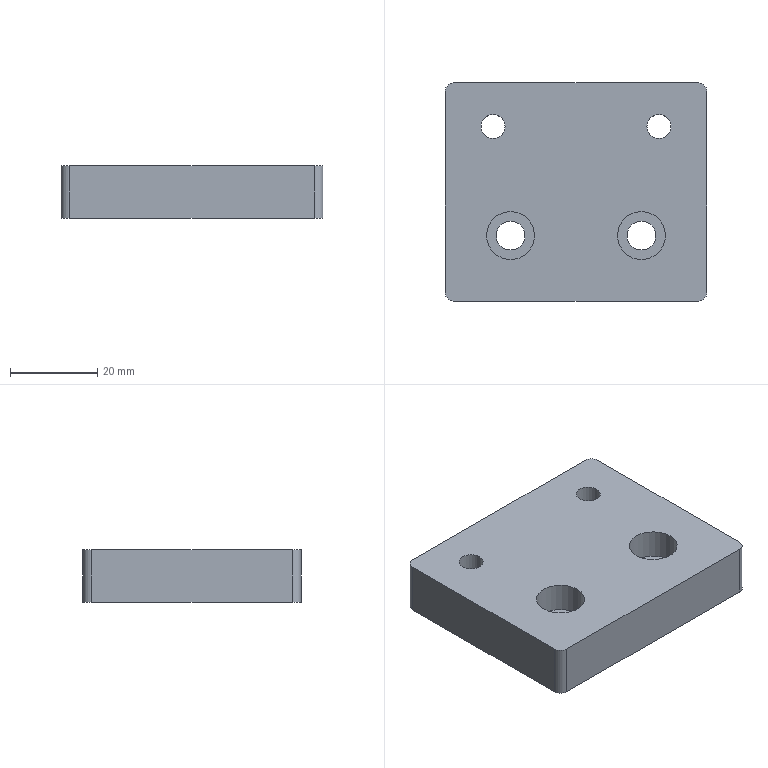Part | STEP file | SynoNew-0304-049 | 1 solid | 22 faces | box 60 x 50 x 12 mm | volume 33116 mm3 | cylinder 12 | plane 10 | commonest cylinder face diameters 4 x4 5.5 x2 6.6 x2 10 x2 11 x2
STEP:
#1=CARTESIAN_POINT('',(-28.,-25.,12.));
#2=VERTEX_POINT('',#1);
#3=CARTESIAN_POINT('',(-30.,-23.,12.));
#4=VERTEX_POINT('',#3);
#5=CARTESIAN_POINT('',(-28.,-23.,12.));
#6=DIRECTION('',(0.,0.,-1.));
#7=DIRECTION('',(-0.7071,-0.7071,0.));
#8=AXIS2_PLACEMENT_3D('',#5,#6,#7);
#9=CIRCLE('',#8,2.);
#10=EDGE_CURVE('',#2,#4,#9,.T.);
#11=ORIENTED_EDGE('',*,*,#10,.T.);
#12=CARTESIAN_POINT('',(-30.,-23.,0.));
#13=VERTEX_POINT('',#12);
#14=CARTESIAN_POINT('',(-30.,-23.,0.));
#15=DIRECTION('',(0.,0.,-1.));
#16=VECTOR('',#15,10.);
#17=LINE('',#14,#16);
#18=EDGE_CURVE('',#4,#13,#17,.T.);
#19=ORIENTED_EDGE('',*,*,#18,.T.);
#20=CARTESIAN_POINT('',(-28.,-25.,0.));
#21=VERTEX_POINT('',#20);
#22=CARTESIAN_POINT('',(-28.,-23.,0.));
#23=DIRECTION('',(0.,0.,1.));
#24=DIRECTION('',(-0.7071,-0.7071,0.));
#25=AXIS2_PLACEMENT_3D('',#22,#23,#24);
#26=CIRCLE('',#25,2.);
#27=EDGE_CURVE('',#13,#21,#26,.T.);
#28=ORIENTED_EDGE('',*,*,#27,.T.);
#29=CARTESIAN_POINT('',(-28.,-25.,0.));
#30=DIRECTION('',(0.,0.,1.));
#31=VECTOR('',#30,10.);
#32=LINE('',#29,#31);
#33=EDGE_CURVE('',#21,#2,#32,.T.);
#34=ORIENTED_EDGE('',*,*,#33,.T.);
#35=EDGE_LOOP('',(#11,#19,#28,#34));
#36=FACE_OUTER_BOUND('',#35,.T.);
#37=CARTESIAN_POINT('',(-28.,-23.,0.));
#38=DIRECTION('',(0.,0.,1.));
#39=DIRECTION('',(-0.7071,-0.7071,0.));
#40=AXIS2_PLACEMENT_3D('',#37,#38,#39);
#41=CYLINDRICAL_SURFACE('',#40,2.);
#42=ADVANCED_FACE('',(#36),#41,.T.);
#43=ORIENTED_EDGE('',*,*,#18,.F.);
#44=CARTESIAN_POINT('',(-30.,23.,12.));
#45=VERTEX_POINT('',#44);
#46=CARTESIAN_POINT('',(-30.,25.,12.));
#47=DIRECTION('',(0.,-1.,0.));
#48=VECTOR('',#47,10.);
#49=LINE('',#46,#48);
#50=EDGE_CURVE('',#45,#4,#49,.T.);
#51=ORIENTED_EDGE('',*,*,#50,.F.);
#52=CARTESIAN_POINT('',(-30.,23.,0.));
#53=VERTEX_POINT('',#52);
#54=CARTESIAN_POINT('',(-30.,23.,0.));
#55=DIRECTION('',(0.,0.,1.));
#56=VECTOR('',#55,10.);
#57=LINE('',#54,#56);
#58=EDGE_CURVE('',#53,#45,#57,.T.);
#59=ORIENTED_EDGE('',*,*,#58,.F.);
#60=CARTESIAN_POINT('',(-30.,25.,0.));
#61=DIRECTION('',(0.,-1.,0.));
#62=VECTOR('',#61,10.);
#63=LINE('',#60,#62);
#64=EDGE_CURVE('',#53,#13,#63,.T.);
#65=ORIENTED_EDGE('',*,*,#64,.T.);
#66=EDGE_LOOP('',(#43,#51,#59,#65));
#67=FACE_OUTER_BOUND('',#66,.T.);
#68=CARTESIAN_POINT('',(-30.,25.,0.));
#69=DIRECTION('',(-1.,0.,0.));
#70=DIRECTION('',(0.,-1.,0.));
#71=AXIS2_PLACEMENT_3D('',#68,#69,#70);
#72=PLANE('',#71);
#73=ADVANCED_FACE('',(#67),#72,.T.);
#74=ORIENTED_EDGE('',*,*,#10,.F.);
#75=CARTESIAN_POINT('',(28.,-25.,12.));
#76=VERTEX_POINT('',#75);
#77=CARTESIAN_POINT('',(-30.,-25.,12.));
#78=DIRECTION('',(1.,0.,0.));
#79=VECTOR('',#78,10.);
#80=LINE('',#77,#79);
#81=EDGE_CURVE('',#2,#76,#80,.T.);
#82=ORIENTED_EDGE('',*,*,#81,.T.);
#83=CARTESIAN_POINT('',(30.,-23.,12.));
#84=VERTEX_POINT('',#83);
#85=CARTESIAN_POINT('',(28.,-23.,12.));
#86=DIRECTION('',(0.,0.,-1.));
#87=DIRECTION('',(0.7071,-0.7071,0.));
#88=AXIS2_PLACEMENT_3D('',#85,#86,#87);
#89=CIRCLE('',#88,2.);
#90=EDGE_CURVE('',#84,#76,#89,.T.);
#91=ORIENTED_EDGE('',*,*,#90,.F.);
#92=CARTESIAN_POINT('',(30.,23.,12.));
#93=VERTEX_POINT('',#92);
#94=CARTESIAN_POINT('',(30.,-25.,12.));
#95=DIRECTION('',(0.,1.,0.));
#96=VECTOR('',#95,10.);
#97=LINE('',#94,#96);
#98=EDGE_CURVE('',#84,#93,#97,.T.);
#99=ORIENTED_EDGE('',*,*,#98,.T.);
#100=CARTESIAN_POINT('',(28.,25.,12.));
#101=VERTEX_POINT('',#100);
#102=CARTESIAN_POINT('',(28.,23.,12.));
#103=DIRECTION('',(0.,0.,-1.));
#104=DIRECTION('',(0.7071,0.7071,0.));
#105=AXIS2_PLACEMENT_3D('',#102,#103,#104);
#106=CIRCLE('',#105,2.);
#107=EDGE_CURVE('',#101,#93,#106,.T.);
#108=ORIENTED_EDGE('',*,*,#107,.F.);
#109=CARTESIAN_POINT('',(-28.,25.,12.));
#110=VERTEX_POINT('',#109);
#111=CARTESIAN_POINT('',(30.,25.,12.));
#112=DIRECTION('',(-1.,0.,0.));
#113=VECTOR('',#112,10.);
#114=LINE('',#111,#113);
#115=EDGE_CURVE('',#101,#110,#114,.T.);
#116=ORIENTED_EDGE('',*,*,#115,.T.);
#117=CARTESIAN_POINT('',(-28.,23.,12.));
#118=DIRECTION('',(0.,0.,-1.));
#119=DIRECTION('',(-0.7071,0.7071,0.));
#120=AXIS2_PLACEMENT_3D('',#117,#118,#119);
#121=CIRCLE('',#120,2.);
#122=EDGE_CURVE('',#45,#110,#121,.T.);
#123=ORIENTED_EDGE('',*,*,#122,.F.);
#124=ORIENTED_EDGE('',*,*,#50,.T.);
#125=EDGE_LOOP('',(#74,#82,#91,#99,#108,#116,#123,#124));
#126=FACE_OUTER_BOUND('',#125,.T.);
#127=CARTESIAN_POINT('',(20.5,-10.,12.));
#128=VERTEX_POINT('',#127);
#129=CARTESIAN_POINT('',(9.5,-10.,12.));
#130=VERTEX_POINT('',#129);
#131=CARTESIAN_POINT('',(15.,-10.,12.));
#132=DIRECTION('',(0.,0.,-1.));
#133=DIRECTION('',(1.,0.,0.));
#134=AXIS2_PLACEMENT_3D('',#131,#132,#133);
#135=CIRCLE('',#134,5.5);
#136=EDGE_CURVE('',#128,#130,#135,.T.);
#137=ORIENTED_EDGE('',*,*,#136,.T.);
#138=CARTESIAN_POINT('',(15.,-10.,12.));
#139=DIRECTION('',(0.,0.,-1.));
#140=DIRECTION('',(1.,0.,0.));
#141=AXIS2_PLACEMENT_3D('',#138,#139,#140);
#142=CIRCLE('',#141,5.5);
#143=EDGE_CURVE('',#130,#128,#142,.T.);
#144=ORIENTED_EDGE('',*,*,#143,.T.);
#145=EDGE_LOOP('',(#137,#144));
#146=FACE_BOUND('',#145,.T.);
#147=CARTESIAN_POINT('',(-9.5,-10.,12.));
#148=VERTEX_POINT('',#147);
#149=CARTESIAN_POINT('',(-20.5,-10.,12.));
#150=VERTEX_POINT('',#149);
#151=CARTESIAN_POINT('',(-15.,-10.,12.));
#152=DIRECTION('',(0.,0.,-1.));
#153=DIRECTION('',(1.,0.,0.));
#154=AXIS2_PLACEMENT_3D('',#151,#152,#153);
#155=CIRCLE('',#154,5.5);
#156=EDGE_CURVE('',#148,#150,#155,.T.);
#157=ORIENTED_EDGE('',*,*,#156,.T.);
#158=CARTESIAN_POINT('',(-15.,-10.,12.));
#159=DIRECTION('',(0.,0.,-1.));
#160=DIRECTION('',(1.,0.,0.));
#161=AXIS2_PLACEMENT_3D('',#158,#159,#160);
#162=CIRCLE('',#161,5.5);
#163=EDGE_CURVE('',#150,#148,#162,.T.);
#164=ORIENTED_EDGE('',*,*,#163,.T.);
#165=EDGE_LOOP('',(#157,#164));
#166=FACE_BOUND('',#165,.T.);
#167=CARTESIAN_POINT('',(-16.25,15.,12.));
#168=VERTEX_POINT('',#167);
#169=CARTESIAN_POINT('',(-19.,15.,12.));
#170=DIRECTION('',(0.,0.,-1.));
#171=DIRECTION('',(-1.,0.,0.));
#172=AXIS2_PLACEMENT_3D('',#169,#170,#171);
#173=CIRCLE('',#172,2.75);
#174=EDGE_CURVE('',#168,#168,#173,.T.);
#175=ORIENTED_EDGE('',*,*,#174,.T.);
#176=EDGE_LOOP('',(#175));
#177=FACE_BOUND('',#176,.T.);
#178=CARTESIAN_POINT('',(21.75,15.,12.));
#179=VERTEX_POINT('',#178);
#180=CARTESIAN_POINT('',(19.,15.,12.));
#181=DIRECTION('',(0.,0.,-1.));
#182=DIRECTION('',(-1.,0.,0.));
#183=AXIS2_PLACEMENT_3D('',#180,#181,#182);
#184=CIRCLE('',#183,2.75);
#185=EDGE_CURVE('',#179,#179,#184,.T.);
#186=ORIENTED_EDGE('',*,*,#185,.T.);
#187=EDGE_LOOP('',(#186));
#188=FACE_BOUND('',#187,.T.);
#189=CARTESIAN_POINT('',(0.,0.,12.));
#190=DIRECTION('',(0.,0.,1.));
#191=DIRECTION('',(1.,0.,0.));
#192=AXIS2_PLACEMENT_3D('',#189,#190,#191);
#193=PLANE('',#192);
#194=ADVANCED_FACE('',(#126,#146,#166,#177,#188),#193,.T.);
#195=ORIENTED_EDGE('',*,*,#90,.T.);
#196=CARTESIAN_POINT('',(28.,-25.,0.));
#197=VERTEX_POINT('',#196);
#198=CARTESIAN_POINT('',(28.,-25.,0.));
#199=DIRECTION('',(0.,0.,-1.));
#200=VECTOR('',#199,10.);
#201=LINE('',#198,#200);
#202=EDGE_CURVE('',#76,#197,#201,.T.);
#203=ORIENTED_EDGE('',*,*,#202,.T.);
#204=CARTESIAN_POINT('',(30.,-23.,0.));
#205=VERTEX_POINT('',#204);
#206=CARTESIAN_POINT('',(28.,-23.,0.));
#207=DIRECTION('',(0.,0.,1.));
#208=DIRECTION('',(0.7071,-0.7071,0.));
#209=AXIS2_PLACEMENT_3D('',#206,#207,#208);
#210=CIRCLE('',#209,2.);
#211=EDGE_CURVE('',#197,#205,#210,.T.);
#212=ORIENTED_EDGE('',*,*,#211,.T.);
#213=CARTESIAN_POINT('',(30.,-23.,0.));
#214=DIRECTION('',(0.,0.,1.));
#215=VECTOR('',#214,10.);
#216=LINE('',#213,#215);
#217=EDGE_CURVE('',#205,#84,#216,.T.);
#218=ORIENTED_EDGE('',*,*,#217,.T.);
#219=EDGE_LOOP('',(#195,#203,#212,#218));
#220=FACE_OUTER_BOUND('',#219,.T.);
#221=CARTESIAN_POINT('',(28.,-23.,0.));
#222=DIRECTION('',(0.,0.,1.));
#223=DIRECTION('',(0.7071,-0.7071,0.));
#224=AXIS2_PLACEMENT_3D('',#221,#222,#223);
#225=CYLINDRICAL_SURFACE('',#224,2.);
#226=ADVANCED_FACE('',(#220),#225,.T.);
#227=ORIENTED_EDGE('',*,*,#217,.F.);
#228=CARTESIAN_POINT('',(30.,23.,0.));
#229=VERTEX_POINT('',#228);
#230=CARTESIAN_POINT('',(30.,-25.,0.));
#231=DIRECTION('',(0.,1.,0.));
#232=VECTOR('',#231,10.);
#233=LINE('',#230,#232);
#234=EDGE_CURVE('',#205,#229,#233,.T.);
#235=ORIENTED_EDGE('',*,*,#234,.T.);
#236=CARTESIAN_POINT('',(30.,23.,0.));
#237=DIRECTION('',(0.,0.,-1.));
#238=VECTOR('',#237,10.);
#239=LINE('',#236,#238);
#240=EDGE_CURVE('',#93,#229,#239,.T.);
#241=ORIENTED_EDGE('',*,*,#240,.F.);
#242=ORIENTED_EDGE('',*,*,#98,.F.);
#243=EDGE_LOOP('',(#227,#235,#241,#242));
#244=FACE_OUTER_BOUND('',#243,.T.);
#245=CARTESIAN_POINT('',(30.,-25.,0.));
#246=DIRECTION('',(1.,0.,0.));
#247=DIRECTION('',(0.,1.,0.));
#248=AXIS2_PLACEMENT_3D('',#245,#246,#247);
#249=PLANE('',#248);
#250=ADVANCED_FACE('',(#244),#249,.T.);
#251=ORIENTED_EDGE('',*,*,#107,.T.);
#252=ORIENTED_EDGE('',*,*,#240,.T.);
#253=CARTESIAN_POINT('',(28.,25.,0.));
#254=VERTEX_POINT('',#253);
#255=CARTESIAN_POINT('',(28.,23.,0.));
#256=DIRECTION('',(0.,0.,1.));
#257=DIRECTION('',(0.7071,0.7071,0.));
#258=AXIS2_PLACEMENT_3D('',#255,#256,#257);
#259=CIRCLE('',#258,2.);
#260=EDGE_CURVE('',#229,#254,#259,.T.);
#261=ORIENTED_EDGE('',*,*,#260,.T.);
#262=CARTESIAN_POINT('',(28.,25.,0.));
#263=DIRECTION('',(0.,0.,1.));
#264=VECTOR('',#263,10.);
#265=LINE('',#262,#264);
#266=EDGE_CURVE('',#254,#101,#265,.T.);
#267=ORIENTED_EDGE('',*,*,#266,.T.);
#268=EDGE_LOOP('',(#251,#252,#261,#267));
#269=FACE_OUTER_BOUND('',#268,.T.);
#270=CARTESIAN_POINT('',(28.,23.,0.));
#271=DIRECTION('',(0.,0.,1.));
#272=DIRECTION('',(0.7071,0.7071,0.));
#273=AXIS2_PLACEMENT_3D('',#270,#271,#272);
#274=CYLINDRICAL_SURFACE('',#273,2.);
#275=ADVANCED_FACE('',(#269),#274,.T.);
#276=ORIENTED_EDGE('',*,*,#122,.T.);
#277=CARTESIAN_POINT('',(-28.,25.,0.));
#278=VERTEX_POINT('',#277);
#279=CARTESIAN_POINT('',(-28.,25.,0.));
#280=DIRECTION('',(0.,0.,-1.));
#281=VECTOR('',#280,10.);
#282=LINE('',#279,#281);
#283=EDGE_CURVE('',#110,#278,#282,.T.);
#284=ORIENTED_EDGE('',*,*,#283,.T.);
#285=CARTESIAN_POINT('',(-28.,23.,0.));
#286=DIRECTION('',(0.,0.,1.));
#287=DIRECTION('',(-0.7071,0.7071,0.));
#288=AXIS2_PLACEMENT_3D('',#285,#286,#287);
#289=CIRCLE('',#288,2.);
#290=EDGE_CURVE('',#278,#53,#289,.T.);
#291=ORIENTED_EDGE('',*,*,#290,.T.);
#292=ORIENTED_EDGE('',*,*,#58,.T.);
#293=EDGE_LOOP('',(#276,#284,#291,#292));
#294=FACE_OUTER_BOUND('',#293,.T.);
#295=CARTESIAN_POINT('',(-28.,23.,0.));
#296=DIRECTION('',(0.,0.,1.));
#297=DIRECTION('',(-0.7071,0.7071,0.));
#298=AXIS2_PLACEMENT_3D('',#295,#296,#297);
#299=CYLINDRICAL_SURFACE('',#298,2.);
#300=ADVANCED_FACE('',(#294),#299,.T.);
#301=CARTESIAN_POINT('',(20.5,-10.,5.2));
#302=VERTEX_POINT('',#301);
#303=CARTESIAN_POINT('',(9.5,-10.,5.2));
#304=VERTEX_POINT('',#303);
#305=CARTESIAN_POINT('',(15.,-10.,5.2));
#306=DIRECTION('',(0.,0.,1.));
#307=DIRECTION('',(1.,0.,0.));
#308=AXIS2_PLACEMENT_3D('',#305,#306,#307);
#309=CIRCLE('',#308,5.5);
#310=EDGE_CURVE('',#302,#304,#309,.T.);
#311=ORIENTED_EDGE('',*,*,#310,.T.);
#312=CARTESIAN_POINT('',(15.,-10.,5.2));
#313=DIRECTION('',(0.,0.,1.));
#314=DIRECTION('',(1.,0.,0.));
#315=AXIS2_PLACEMENT_3D('',#312,#313,#314);
#316=CIRCLE('',#315,5.5);
#317=EDGE_CURVE('',#304,#302,#316,.T.);
#318=ORIENTED_EDGE('',*,*,#317,.T.);
#319=EDGE_LOOP('',(#311,#318));
#320=FACE_OUTER_BOUND('',#319,.T.);
#321=CARTESIAN_POINT('',(11.7,-10.,5.2));
#322=VERTEX_POINT('',#321);
#323=CARTESIAN_POINT('',(15.,-10.,5.2));
#324=DIRECTION('',(0.,0.,1.));
#325=DIRECTION('',(1.,0.,0.));
#326=AXIS2_PLACEMENT_3D('',#323,#324,#325);
#327=CIRCLE('',#326,3.3);
#328=EDGE_CURVE('',#322,#322,#327,.T.);
#329=ORIENTED_EDGE('',*,*,#328,.F.);
#330=EDGE_LOOP('',(#329));
#331=FACE_BOUND('',#330,.T.);
#332=CARTESIAN_POINT('',(15.,-10.,5.2));
#333=DIRECTION('',(0.,0.,1.));
#334=DIRECTION('',(1.,0.,0.));
#335=AXIS2_PLACEMENT_3D('',#332,#333,#334);
#336=PLANE('',#335);
#337=ADVANCED_FACE('',(#320,#331),#336,.T.);
#338=ORIENTED_EDGE('',*,*,#136,.F.);
#339=ORIENTED_EDGE('',*,*,#143,.F.);
#340=CARTESIAN_POINT('',(9.5,-10.,8.6));
#341=DIRECTION('',(0.,0.,-1.));
#342=VECTOR('',#341,5.5);
#343=LINE('',#340,#342);
#344=EDGE_CURVE('',#130,#304,#343,.T.);
#345=ORIENTED_EDGE('',*,*,#344,.T.);
#346=ORIENTED_EDGE('',*,*,#310,.F.);
#347=ORIENTED_EDGE('',*,*,#317,.F.);
#348=ORIENTED_EDGE('',*,*,#344,.F.);
#349=EDGE_LOOP('',(#338,#339,#345,#346,#347,#348));
#350=FACE_OUTER_BOUND('',#349,.T.);
#351=CARTESIAN_POINT('',(15.,-10.,8.6));
#352=DIRECTION('',(0.,0.,1.));
#353=DIRECTION('',(1.,0.,0.));
#354=AXIS2_PLACEMENT_3D('',#351,#352,#353);
#355=CYLINDRICAL_SURFACE('',#354,5.5);
#356=ADVANCED_FACE('',(#350),#355,.F.);
#357=ORIENTED_EDGE('',*,*,#328,.T.);
#358=CARTESIAN_POINT('',(11.7,-10.,0.));
#359=VERTEX_POINT('',#358);
#360=CARTESIAN_POINT('',(11.7,-10.,-67.019));
#361=DIRECTION('',(0.,0.,-1.));
#362=VECTOR('',#361,3.3);
#363=LINE('',#360,#362);
#364=EDGE_CURVE('',#322,#359,#363,.T.);
#365=ORIENTED_EDGE('',*,*,#364,.T.);
#366=CARTESIAN_POINT('',(15.,-10.,0.));
#367=DIRECTION('',(0.,0.,1.));
#368=DIRECTION('',(1.,0.,0.));
#369=AXIS2_PLACEMENT_3D('',#366,#367,#368);
#370=CIRCLE('',#369,3.3);
#371=EDGE_CURVE('',#359,#359,#370,.T.);
#372=ORIENTED_EDGE('',*,*,#371,.F.);
#373=ORIENTED_EDGE('',*,*,#364,.F.);
#374=EDGE_LOOP('',(#357,#365,#372,#373));
#375=FACE_OUTER_BOUND('',#374,.T.);
#376=CARTESIAN_POINT('',(15.,-10.,-67.019));
#377=DIRECTION('',(0.,0.,1.));
#378=DIRECTION('',(1.,0.,0.));
#379=AXIS2_PLACEMENT_3D('',#376,#377,#378);
#380=CYLINDRICAL_SURFACE('',#379,3.3);
#381=ADVANCED_FACE('',(#375),#380,.F.);
#382=CARTESIAN_POINT('',(-9.5,-10.,5.2));
#383=VERTEX_POINT('',#382);
#384=CARTESIAN_POINT('',(-20.5,-10.,5.2));
#385=VERTEX_POINT('',#384);
#386=CARTESIAN_POINT('',(-15.,-10.,5.2));
#387=DIRECTION('',(0.,0.,1.));
#388=DIRECTION('',(1.,0.,0.));
#389=AXIS2_PLACEMENT_3D('',#386,#387,#388);
#390=CIRCLE('',#389,5.5);
#391=EDGE_CURVE('',#383,#385,#390,.T.);
#392=ORIENTED_EDGE('',*,*,#391,.T.);
#393=CARTESIAN_POINT('',(-15.,-10.,5.2));
#394=DIRECTION('',(0.,0.,1.));
#395=DIRECTION('',(1.,0.,0.));
#396=AXIS2_PLACEMENT_3D('',#393,#394,#395);
#397=CIRCLE('',#396,5.5);
#398=EDGE_CURVE('',#385,#383,#397,.T.);
#399=ORIENTED_EDGE('',*,*,#398,.T.);
#400=EDGE_LOOP('',(#392,#399));
#401=FACE_OUTER_BOUND('',#400,.T.);
#402=CARTESIAN_POINT('',(-18.3,-10.,5.2));
#403=VERTEX_POINT('',#402);
#404=CARTESIAN_POINT('',(-15.,-10.,5.2));
#405=DIRECTION('',(0.,0.,1.));
#406=DIRECTION('',(1.,0.,0.));
#407=AXIS2_PLACEMENT_3D('',#404,#405,#406);
#408=CIRCLE('',#407,3.3);
#409=EDGE_CURVE('',#403,#403,#408,.T.);
#410=ORIENTED_EDGE('',*,*,#409,.F.);
#411=EDGE_LOOP('',(#410));
#412=FACE_BOUND('',#411,.T.);
#413=CARTESIAN_POINT('',(-15.,-10.,5.2));
#414=DIRECTION('',(0.,0.,1.));
#415=DIRECTION('',(1.,0.,0.));
#416=AXIS2_PLACEMENT_3D('',#413,#414,#415);
#417=PLANE('',#416);
#418=ADVANCED_FACE('',(#401,#412),#417,.T.);
#419=ORIENTED_EDGE('',*,*,#156,.F.);
#420=ORIENTED_EDGE('',*,*,#163,.F.);
#421=CARTESIAN_POINT('',(-20.5,-10.,8.6));
#422=DIRECTION('',(0.,0.,-1.));
#423=VECTOR('',#422,5.5);
#424=LINE('',#421,#423);
#425=EDGE_CURVE('',#150,#385,#424,.T.);
#426=ORIENTED_EDGE('',*,*,#425,.T.);
#427=ORIENTED_EDGE('',*,*,#391,.F.);
#428=ORIENTED_EDGE('',*,*,#398,.F.);
#429=ORIENTED_EDGE('',*,*,#425,.F.);
#430=EDGE_LOOP('',(#419,#420,#426,#427,#428,#429));
#431=FACE_OUTER_BOUND('',#430,.T.);
#432=CARTESIAN_POINT('',(-15.,-10.,8.6));
#433=DIRECTION('',(0.,0.,1.));
#434=DIRECTION('',(1.,0.,0.));
#435=AXIS2_PLACEMENT_3D('',#432,#433,#434);
#436=CYLINDRICAL_SURFACE('',#435,5.5);
#437=ADVANCED_FACE('',(#431),#436,.F.);
#438=ORIENTED_EDGE('',*,*,#409,.T.);
#439=CARTESIAN_POINT('',(-18.3,-10.,0.));
#440=VERTEX_POINT('',#439);
#441=CARTESIAN_POINT('',(-18.3,-10.,-67.019));
#442=DIRECTION('',(0.,0.,-1.));
#443=VECTOR('',#442,3.3);
#444=LINE('',#441,#443);
#445=EDGE_CURVE('',#403,#440,#444,.T.);
#446=ORIENTED_EDGE('',*,*,#445,.T.);
#447=CARTESIAN_POINT('',(-15.,-10.,0.));
#448=DIRECTION('',(0.,0.,1.));
#449=DIRECTION('',(1.,0.,0.));
#450=AXIS2_PLACEMENT_3D('',#447,#448,#449);
#451=CIRCLE('',#450,3.3);
#452=EDGE_CURVE('',#440,#440,#451,.T.);
#453=ORIENTED_EDGE('',*,*,#452,.F.);
#454=ORIENTED_EDGE('',*,*,#445,.F.);
#455=EDGE_LOOP('',(#438,#446,#453,#454));
#456=FACE_OUTER_BOUND('',#455,.T.);
#457=CARTESIAN_POINT('',(-15.,-10.,-67.019));
#458=DIRECTION('',(0.,0.,1.));
#459=DIRECTION('',(1.,0.,0.));
#460=AXIS2_PLACEMENT_3D('',#457,#458,#459);
#461=CYLINDRICAL_SURFACE('',#460,3.3);
#462=ADVANCED_FACE('',(#456),#461,.F.);
#463=CARTESIAN_POINT('',(-24.,15.,5.7));
#464=VERTEX_POINT('',#463);
#465=CARTESIAN_POINT('',(-14.,15.,5.7));
#466=VERTEX_POINT('',#465);
#467=CARTESIAN_POINT('',(-19.,15.,5.7));
#468=DIRECTION('',(0.,0.,-1.));
#469=DIRECTION('',(-1.,0.,0.));
#470=AXIS2_PLACEMENT_3D('',#467,#468,#469);
#471=CIRCLE('',#470,5.);
#472=EDGE_CURVE('',#464,#466,#471,.T.);
#473=ORIENTED_EDGE('',*,*,#472,.T.);
#474=CARTESIAN_POINT('',(-19.,15.,5.7));
#475=DIRECTION('',(0.,0.,-1.));
#476=DIRECTION('',(-1.,0.,0.));
#477=AXIS2_PLACEMENT_3D('',#474,#475,#476);
#478=CIRCLE('',#477,5.);
#479=EDGE_CURVE('',#466,#464,#478,.T.);
#480=ORIENTED_EDGE('',*,*,#479,.T.);
#481=EDGE_LOOP('',(#473,#480));
#482=FACE_OUTER_BOUND('',#481,.T.);
#483=CARTESIAN_POINT('',(-16.25,15.,5.7));
#484=VERTEX_POINT('',#483);
#485=CARTESIAN_POINT('',(-19.,15.,5.7));
#486=DIRECTION('',(0.,0.,-1.));
#487=DIRECTION('',(-1.,0.,0.));
#488=AXIS2_PLACEMENT_3D('',#485,#486,#487);
#489=CIRCLE('',#488,2.75);
#490=EDGE_CURVE('',#484,#484,#489,.T.);
#491=ORIENTED_EDGE('',*,*,#490,.F.);
#492=EDGE_LOOP('',(#491));
#493=FACE_BOUND('',#492,.T.);
#494=CARTESIAN_POINT('',(-19.,15.,5.7));
#495=DIRECTION('',(0.,0.,-1.));
#496=DIRECTION('',(-1.,0.,0.));
#497=AXIS2_PLACEMENT_3D('',#494,#495,#496);
#498=PLANE('',#497);
#499=ADVANCED_FACE('',(#482,#493),#498,.T.);
#500=CARTESIAN_POINT('',(-24.,15.,0.));
#501=VERTEX_POINT('',#500);
#502=CARTESIAN_POINT('',(-14.,15.,0.));
#503=VERTEX_POINT('',#502);
#504=CARTESIAN_POINT('',(-19.,15.,0.));
#505=DIRECTION('',(0.,0.,1.));
#506=DIRECTION('',(-1.,0.,0.));
#507=AXIS2_PLACEMENT_3D('',#504,#505,#506);
#508=CIRCLE('',#507,5.);
#509=EDGE_CURVE('',#501,#503,#508,.T.);
#510=ORIENTED_EDGE('',*,*,#509,.F.);
#511=CARTESIAN_POINT('',(-19.,15.,0.));
#512=DIRECTION('',(0.,0.,1.));
#513=DIRECTION('',(-1.,0.,0.));
#514=AXIS2_PLACEMENT_3D('',#511,#512,#513);
#515=CIRCLE('',#514,5.);
#516=EDGE_CURVE('',#503,#501,#515,.T.);
#517=ORIENTED_EDGE('',*,*,#516,.F.);
#518=CARTESIAN_POINT('',(-14.,15.,2.85));
#519=DIRECTION('',(0.,0.,1.));
#520=VECTOR('',#519,5.);
#521=LINE('',#518,#520);
#522=EDGE_CURVE('',#503,#466,#521,.T.);
#523=ORIENTED_EDGE('',*,*,#522,.T.);
#524=ORIENTED_EDGE('',*,*,#472,.F.);
#525=ORIENTED_EDGE('',*,*,#479,.F.);
#526=ORIENTED_EDGE('',*,*,#522,.F.);
#527=EDGE_LOOP('',(#510,#517,#523,#524,#525,#526));
#528=FACE_OUTER_BOUND('',#527,.T.);
#529=CARTESIAN_POINT('',(-19.,15.,2.85));
#530=DIRECTION('',(0.,0.,-1.));
#531=DIRECTION('',(-1.,0.,0.));
#532=AXIS2_PLACEMENT_3D('',#529,#530,#531);
#533=CYLINDRICAL_SURFACE('',#532,5.);
#534=ADVANCED_FACE('',(#528),#533,.F.);
#535=ORIENTED_EDGE('',*,*,#490,.T.);
#536=CARTESIAN_POINT('',(-16.25,15.,79.019));
#537=DIRECTION('',(0.,0.,1.));
#538=VECTOR('',#537,2.75);
#539=LINE('',#536,#538);
#540=EDGE_CURVE('',#484,#168,#539,.T.);
#541=ORIENTED_EDGE('',*,*,#540,.T.);
#542=ORIENTED_EDGE('',*,*,#174,.F.);
#543=ORIENTED_EDGE('',*,*,#540,.F.);
#544=EDGE_LOOP('',(#535,#541,#542,#543));
#545=FACE_OUTER_BOUND('',#544,.T.);
#546=CARTESIAN_POINT('',(-19.,15.,79.019));
#547=DIRECTION('',(0.,0.,-1.));
#548=DIRECTION('',(-1.,0.,0.));
#549=AXIS2_PLACEMENT_3D('',#546,#547,#548);
#550=CYLINDRICAL_SURFACE('',#549,2.75);
#551=ADVANCED_FACE('',(#545),#550,.F.);
#552=CARTESIAN_POINT('',(14.,15.,5.7));
#553=VERTEX_POINT('',#552);
#554=CARTESIAN_POINT('',(24.,15.,5.7));
#555=VERTEX_POINT('',#554);
#556=CARTESIAN_POINT('',(19.,15.,5.7));
#557=DIRECTION('',(0.,0.,-1.));
#558=DIRECTION('',(-1.,0.,0.));
#559=AXIS2_PLACEMENT_3D('',#556,#557,#558);
#560=CIRCLE('',#559,5.);
#561=EDGE_CURVE('',#553,#555,#560,.T.);
#562=ORIENTED_EDGE('',*,*,#561,.T.);
#563=CARTESIAN_POINT('',(19.,15.,5.7));
#564=DIRECTION('',(0.,0.,-1.));
#565=DIRECTION('',(-1.,0.,0.));
#566=AXIS2_PLACEMENT_3D('',#563,#564,#565);
#567=CIRCLE('',#566,5.);
#568=EDGE_CURVE('',#555,#553,#567,.T.);
#569=ORIENTED_EDGE('',*,*,#568,.T.);
#570=EDGE_LOOP('',(#562,#569));
#571=FACE_OUTER_BOUND('',#570,.T.);
#572=CARTESIAN_POINT('',(21.75,15.,5.7));
#573=VERTEX_POINT('',#572);
#574=CARTESIAN_POINT('',(19.,15.,5.7));
#575=DIRECTION('',(0.,0.,-1.));
#576=DIRECTION('',(-1.,0.,0.));
#577=AXIS2_PLACEMENT_3D('',#574,#575,#576);
#578=CIRCLE('',#577,2.75);
#579=EDGE_CURVE('',#573,#573,#578,.T.);
#580=ORIENTED_EDGE('',*,*,#579,.F.);
#581=EDGE_LOOP('',(#580));
#582=FACE_BOUND('',#581,.T.);
#583=CARTESIAN_POINT('',(19.,15.,5.7));
#584=DIRECTION('',(0.,0.,-1.));
#585=DIRECTION('',(-1.,0.,0.));
#586=AXIS2_PLACEMENT_3D('',#583,#584,#585);
#587=PLANE('',#586);
#588=ADVANCED_FACE('',(#571,#582),#587,.T.);
#589=CARTESIAN_POINT('',(14.,15.,0.));
#590=VERTEX_POINT('',#589);
#591=CARTESIAN_POINT('',(24.,15.,0.));
#592=VERTEX_POINT('',#591);
#593=CARTESIAN_POINT('',(19.,15.,0.));
#594=DIRECTION('',(0.,0.,1.));
#595=DIRECTION('',(-1.,0.,0.));
#596=AXIS2_PLACEMENT_3D('',#593,#594,#595);
#597=CIRCLE('',#596,5.);
#598=EDGE_CURVE('',#590,#592,#597,.T.);
#599=ORIENTED_EDGE('',*,*,#598,.F.);
#600=CARTESIAN_POINT('',(19.,15.,0.));
#601=DIRECTION('',(0.,0.,1.));
#602=DIRECTION('',(-1.,0.,0.));
#603=AXIS2_PLACEMENT_3D('',#600,#601,#602);
#604=CIRCLE('',#603,5.);
#605=EDGE_CURVE('',#592,#590,#604,.T.);
#606=ORIENTED_EDGE('',*,*,#605,.F.);
#607=CARTESIAN_POINT('',(24.,15.,2.85));
#608=DIRECTION('',(0.,0.,1.));
#609=VECTOR('',#608,5.);
#610=LINE('',#607,#609);
#611=EDGE_CURVE('',#592,#555,#610,.T.);
#612=ORIENTED_EDGE('',*,*,#611,.T.);
#613=ORIENTED_EDGE('',*,*,#561,.F.);
#614=ORIENTED_EDGE('',*,*,#568,.F.);
#615=ORIENTED_EDGE('',*,*,#611,.F.);
#616=EDGE_LOOP('',(#599,#606,#612,#613,#614,#615));
#617=FACE_OUTER_BOUND('',#616,.T.);
#618=CARTESIAN_POINT('',(19.,15.,2.85));
#619=DIRECTION('',(0.,0.,-1.));
#620=DIRECTION('',(-1.,0.,0.));
#621=AXIS2_PLACEMENT_3D('',#618,#619,#620);
#622=CYLINDRICAL_SURFACE('',#621,5.);
#623=ADVANCED_FACE('',(#617),#622,.F.);
#624=ORIENTED_EDGE('',*,*,#579,.T.);
#625=CARTESIAN_POINT('',(21.75,15.,79.019));
#626=DIRECTION('',(0.,0.,1.));
#627=VECTOR('',#626,2.75);
#628=LINE('',#625,#627);
#629=EDGE_CURVE('',#573,#179,#628,.T.);
#630=ORIENTED_EDGE('',*,*,#629,.T.);
#631=ORIENTED_EDGE('',*,*,#185,.F.);
#632=ORIENTED_EDGE('',*,*,#629,.F.);
#633=EDGE_LOOP('',(#624,#630,#631,#632));
#634=FACE_OUTER_BOUND('',#633,.T.);
#635=CARTESIAN_POINT('',(19.,15.,79.019));
#636=DIRECTION('',(0.,0.,-1.));
#637=DIRECTION('',(-1.,0.,0.));
#638=AXIS2_PLACEMENT_3D('',#635,#636,#637);
#639=CYLINDRICAL_SURFACE('',#638,2.75);
#640=ADVANCED_FACE('',(#634),#639,.F.);
#641=ORIENTED_EDGE('',*,*,#266,.F.);
#642=CARTESIAN_POINT('',(30.,25.,0.));
#643=DIRECTION('',(-1.,0.,0.));
#644=VECTOR('',#643,10.);
#645=LINE('',#642,#644);
#646=EDGE_CURVE('',#254,#278,#645,.T.);
#647=ORIENTED_EDGE('',*,*,#646,.T.);
#648=ORIENTED_EDGE('',*,*,#283,.F.);
#649=ORIENTED_EDGE('',*,*,#115,.F.);
#650=EDGE_LOOP('',(#641,#647,#648,#649));
#651=FACE_OUTER_BOUND('',#650,.T.);
#652=CARTESIAN_POINT('',(30.,25.,0.));
#653=DIRECTION('',(0.,1.,0.));
#654=DIRECTION('',(-1.,0.,0.));
#655=AXIS2_PLACEMENT_3D('',#652,#653,#654);
#656=PLANE('',#655);
#657=ADVANCED_FACE('',(#651),#656,.T.);
#658=ORIENTED_EDGE('',*,*,#33,.F.);
#659=CARTESIAN_POINT('',(-30.,-25.,0.));
#660=DIRECTION('',(1.,0.,0.));
#661=VECTOR('',#660,10.);
#662=LINE('',#659,#661);
#663=EDGE_CURVE('',#21,#197,#662,.T.);
#664=ORIENTED_EDGE('',*,*,#663,.T.);
#665=ORIENTED_EDGE('',*,*,#202,.F.);
#666=ORIENTED_EDGE('',*,*,#81,.F.);
#667=EDGE_LOOP('',(#658,#664,#665,#666));
#668=FACE_OUTER_BOUND('',#667,.T.);
#669=CARTESIAN_POINT('',(-30.,-25.,0.));
#670=DIRECTION('',(0.,-1.,0.));
#671=DIRECTION('',(1.,0.,0.));
#672=AXIS2_PLACEMENT_3D('',#669,#670,#671);
#673=PLANE('',#672);
#674=ADVANCED_FACE('',(#668),#673,.T.);
#675=ORIENTED_EDGE('',*,*,#27,.F.);
#676=ORIENTED_EDGE('',*,*,#64,.F.);
#677=ORIENTED_EDGE('',*,*,#290,.F.);
#678=ORIENTED_EDGE('',*,*,#646,.F.);
#679=ORIENTED_EDGE('',*,*,#260,.F.);
#680=ORIENTED_EDGE('',*,*,#234,.F.);
#681=ORIENTED_EDGE('',*,*,#211,.F.);
#682=ORIENTED_EDGE('',*,*,#663,.F.);
#683=EDGE_LOOP('',(#675,#676,#677,#678,#679,#680,#681,#682));
#684=FACE_OUTER_BOUND('',#683,.T.);
#685=ORIENTED_EDGE('',*,*,#371,.T.);
#686=EDGE_LOOP('',(#685));
#687=FACE_BOUND('',#686,.T.);
#688=ORIENTED_EDGE('',*,*,#452,.T.);
#689=EDGE_LOOP('',(#688));
#690=FACE_BOUND('',#689,.T.);
#691=ORIENTED_EDGE('',*,*,#509,.T.);
#692=ORIENTED_EDGE('',*,*,#516,.T.);
#693=EDGE_LOOP('',(#691,#692));
#694=FACE_BOUND('',#693,.T.);
#695=ORIENTED_EDGE('',*,*,#598,.T.);
#696=ORIENTED_EDGE('',*,*,#605,.T.);
#697=EDGE_LOOP('',(#695,#696));
#698=FACE_BOUND('',#697,.T.);
#699=CARTESIAN_POINT('',(0.,0.,0.));
#700=DIRECTION('',(0.,0.,1.));
#701=DIRECTION('',(1.,0.,0.));
#702=AXIS2_PLACEMENT_3D('',#699,#700,#701);
#703=PLANE('',#702);
#704=ADVANCED_FACE('',(#684,#687,#690,#694,#698),#703,.F.);
#705=CLOSED_SHELL('',(#42,#73,#194,#226,#250,#275,#300,#337,#356,#381,#418,#437,#462,#499,#534,#551,#588,#623,#640,#657,#674,#704));
#706=MANIFOLD_SOLID_BREP('',#705);
#707=(LENGTH_UNIT()NAMED_UNIT(*)SI_UNIT(.MILLI.,.METRE.));
#708=UNCERTAINTY_MEASURE_WITH_UNIT(LENGTH_MEASURE(0.01),#707,'','');
#709=(NAMED_UNIT(*)PLANE_ANGLE_UNIT()SI_UNIT($,.RADIAN.));
#710=(NAMED_UNIT(*)SI_UNIT($,.STERADIAN.)SOLID_ANGLE_UNIT());
#711=(GEOMETRIC_REPRESENTATION_CONTEXT(3)GLOBAL_UNCERTAINTY_ASSIGNED_CONTEXT((#708))GLOBAL_UNIT_ASSIGNED_CONTEXT((#707,#709,#710))REPRESENTATION_CONTEXT('',''));
#712=ADVANCED_BREP_SHAPE_REPRESENTATION('',(#706),#711);